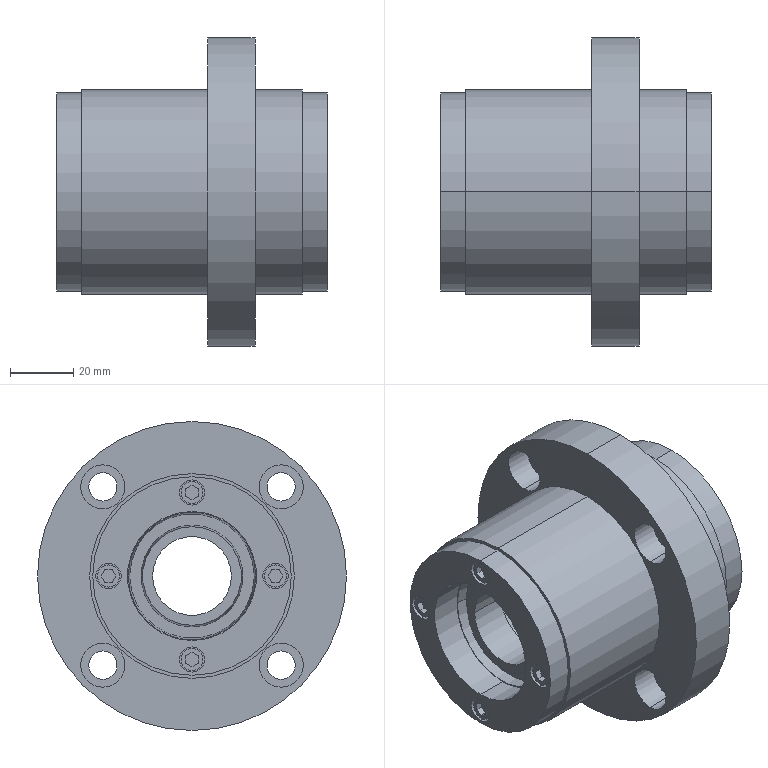Part | SolidWorks | features BaseBody 5 | 5 solids | 300 faces | box 86 x 98 x 98 mm | volume 237483 mm3 | cylinder 128 | plane 124 | cone 48 | commonest cylinder face diameters 2.013 x16 3 x16 4.5 x16 7 x16 8 x16 47 x12